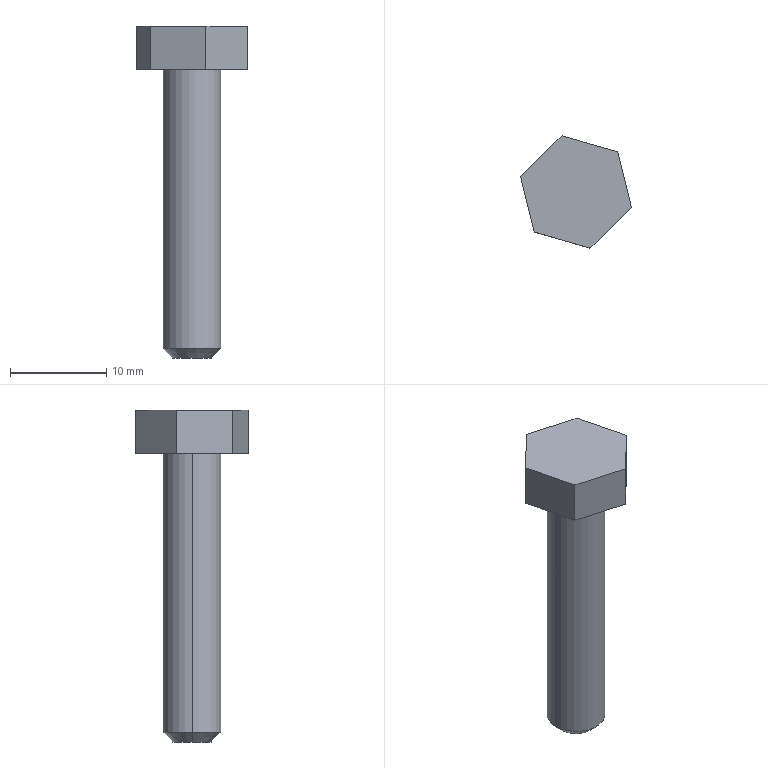Part | SolidWorks | features ICE 2, Chamfer 1, Extrusion 1 | 1 solid | 13 faces | box 11.534 x 11.645 x 34.5 mm | volume 1261 mm3 | plane 9 | cone 2 | cylinder 2 | commonest cylinder face diameters 6 x2
STEP:
#1=CARTESIAN_POINT('',(-2.,0.,-30.));
#2=VERTEX_POINT('',#1);
#3=CARTESIAN_POINT('',(2.,0.,-30.));
#4=VERTEX_POINT('',#3);
#5=CARTESIAN_POINT('',(0.,0.,-30.));
#6=DIRECTION('',(0.,0.,-1.));
#7=DIRECTION('',(-1.,0.,0.));
#8=AXIS2_PLACEMENT_3D('',#5,#6,#7);
#9=CIRCLE('',#8,2.);
#10=EDGE_CURVE('',#2,#4,#9,.T.);
#11=ORIENTED_EDGE('',*,*,#10,.F.);
#12=CARTESIAN_POINT('',(-3.,0.,-29.));
#13=VERTEX_POINT('',#12);
#14=CARTESIAN_POINT('',(-2.,0.,-30.));
#15=DIRECTION('',(-0.7071,0.,0.7071));
#16=VECTOR('',#15,1000.);
#17=LINE('',#14,#16);
#18=EDGE_CURVE('',#2,#13,#17,.T.);
#19=ORIENTED_EDGE('',*,*,#18,.T.);
#20=CARTESIAN_POINT('',(3.,0.,-29.));
#21=VERTEX_POINT('',#20);
#22=CARTESIAN_POINT('',(0.,0.,-29.));
#23=DIRECTION('',(0.,0.,1.));
#24=DIRECTION('',(-1.,0.,0.));
#25=AXIS2_PLACEMENT_3D('',#22,#23,#24);
#26=CIRCLE('',#25,3.);
#27=EDGE_CURVE('',#21,#13,#26,.T.);
#28=ORIENTED_EDGE('',*,*,#27,.F.);
#29=CARTESIAN_POINT('',(2.,0.,-30.));
#30=DIRECTION('',(0.7071,0.,0.7071));
#31=VECTOR('',#30,1000.);
#32=LINE('',#29,#31);
#33=EDGE_CURVE('',#4,#21,#32,.T.);
#34=ORIENTED_EDGE('',*,*,#33,.F.);
#35=EDGE_LOOP('',(#11,#19,#28,#34));
#36=FACE_OUTER_BOUND('',#35,.T.);
#37=CARTESIAN_POINT('',(0.,0.,-30.));
#38=DIRECTION('',(0.,0.,1.));
#39=DIRECTION('',(1.,0.,0.));
#40=AXIS2_PLACEMENT_3D('',#37,#38,#39);
#41=CONICAL_SURFACE('',#40,2.,0.7854);
#42=ADVANCED_FACE('',(#36),#41,.T.);
#43=ORIENTED_EDGE('',*,*,#27,.T.);
#44=CARTESIAN_POINT('',(-3.,0.,0.));
#45=VERTEX_POINT('',#44);
#46=CARTESIAN_POINT('',(-3.,0.,-30.));
#47=DIRECTION('',(0.,0.,1.));
#48=VECTOR('',#47,1000.);
#49=LINE('',#46,#48);
#50=EDGE_CURVE('',#13,#45,#49,.T.);
#51=ORIENTED_EDGE('',*,*,#50,.T.);
#52=CARTESIAN_POINT('',(3.,0.,0.));
#53=VERTEX_POINT('',#52);
#54=CARTESIAN_POINT('',(0.,0.,0.));
#55=DIRECTION('',(0.,0.,-1.));
#56=DIRECTION('',(-1.,0.,0.));
#57=AXIS2_PLACEMENT_3D('',#54,#55,#56);
#58=CIRCLE('',#57,3.);
#59=EDGE_CURVE('',#45,#53,#58,.T.);
#60=ORIENTED_EDGE('',*,*,#59,.T.);
#61=CARTESIAN_POINT('',(3.,0.,-30.));
#62=DIRECTION('',(0.,0.,1.));
#63=VECTOR('',#62,1000.);
#64=LINE('',#61,#63);
#65=EDGE_CURVE('',#21,#53,#64,.T.);
#66=ORIENTED_EDGE('',*,*,#65,.F.);
#67=EDGE_LOOP('',(#43,#51,#60,#66));
#68=FACE_OUTER_BOUND('',#67,.T.);
#69=CARTESIAN_POINT('',(0.,0.,-30.));
#70=DIRECTION('',(0.,0.,1.));
#71=DIRECTION('',(1.,0.,0.));
#72=AXIS2_PLACEMENT_3D('',#69,#70,#71);
#73=CYLINDRICAL_SURFACE('',#72,3.);
#74=ADVANCED_FACE('',(#68),#73,.T.);
#75=CARTESIAN_POINT('',(0.,0.,0.));
#76=DIRECTION('',(0.,0.,-1.));
#77=DIRECTION('',(-1.,0.,0.));
#78=AXIS2_PLACEMENT_3D('',#75,#76,#77);
#79=CIRCLE('',#78,3.);
#80=EDGE_CURVE('',#53,#45,#79,.T.);
#81=ORIENTED_EDGE('',*,*,#80,.F.);
#82=ORIENTED_EDGE('',*,*,#59,.F.);
#83=EDGE_LOOP('',(#81,#82));
#84=FACE_BOUND('',#83,.T.);
#85=CARTESIAN_POINT('',(1.449,-5.822,0.));
#86=VERTEX_POINT('',#85);
#87=CARTESIAN_POINT('',(-4.318,-4.166,0.));
#88=VERTEX_POINT('',#87);
#89=CARTESIAN_POINT('',(1.449,-5.822,0.));
#90=DIRECTION('',(-0.9612,0.276,0.));
#91=VECTOR('',#90,1000.);
#92=LINE('',#89,#91);
#93=EDGE_CURVE('',#86,#88,#92,.T.);
#94=ORIENTED_EDGE('',*,*,#93,.T.);
#95=CARTESIAN_POINT('',(-5.767,1.656,0.));
#96=VERTEX_POINT('',#95);
#97=CARTESIAN_POINT('',(-4.318,-4.166,0.));
#98=DIRECTION('',(-0.2416,0.9704,0.));
#99=VECTOR('',#98,1000.);
#100=LINE('',#97,#99);
#101=EDGE_CURVE('',#88,#96,#100,.T.);
#102=ORIENTED_EDGE('',*,*,#101,.T.);
#103=CARTESIAN_POINT('',(-1.449,5.822,0.));
#104=VERTEX_POINT('',#103);
#105=CARTESIAN_POINT('',(-5.767,1.656,0.));
#106=DIRECTION('',(0.7196,0.6944,0.));
#107=VECTOR('',#106,1000.);
#108=LINE('',#105,#107);
#109=EDGE_CURVE('',#96,#104,#108,.T.);
#110=ORIENTED_EDGE('',*,*,#109,.T.);
#111=CARTESIAN_POINT('',(4.318,4.166,0.));
#112=VERTEX_POINT('',#111);
#113=CARTESIAN_POINT('',(-1.449,5.822,0.));
#114=DIRECTION('',(0.9612,-0.276,0.));
#115=VECTOR('',#114,1000.);
#116=LINE('',#113,#115);
#117=EDGE_CURVE('',#104,#112,#116,.T.);
#118=ORIENTED_EDGE('',*,*,#117,.T.);
#119=CARTESIAN_POINT('',(5.767,-1.656,0.));
#120=VERTEX_POINT('',#119);
#121=CARTESIAN_POINT('',(4.318,4.166,0.));
#122=DIRECTION('',(0.2416,-0.9704,0.));
#123=VECTOR('',#122,1000.);
#124=LINE('',#121,#123);
#125=EDGE_CURVE('',#112,#120,#124,.T.);
#126=ORIENTED_EDGE('',*,*,#125,.T.);
#127=CARTESIAN_POINT('',(5.767,-1.656,0.));
#128=DIRECTION('',(-0.7196,-0.6944,0.));
#129=VECTOR('',#128,1000.);
#130=LINE('',#127,#129);
#131=EDGE_CURVE('',#120,#86,#130,.T.);
#132=ORIENTED_EDGE('',*,*,#131,.T.);
#133=EDGE_LOOP('',(#94,#102,#110,#118,#126,#132));
#134=FACE_OUTER_BOUND('',#133,.T.);
#135=CARTESIAN_POINT('',(0.,0.,0.));
#136=DIRECTION('',(0.,0.,1.));
#137=DIRECTION('',(1.,0.,0.));
#138=AXIS2_PLACEMENT_3D('',#135,#136,#137);
#139=PLANE('',#138);
#140=ADVANCED_FACE('',(#84,#134),#139,.F.);
#141=ORIENTED_EDGE('',*,*,#93,.F.);
#142=CARTESIAN_POINT('',(1.449,-5.822,4.5));
#143=VERTEX_POINT('',#142);
#144=CARTESIAN_POINT('',(1.449,-5.822,4.5));
#145=DIRECTION('',(0.,0.,-1.));
#146=VECTOR('',#145,1000.);
#147=LINE('',#144,#146);
#148=EDGE_CURVE('',#143,#86,#147,.T.);
#149=ORIENTED_EDGE('',*,*,#148,.F.);
#150=CARTESIAN_POINT('',(-4.318,-4.166,4.5));
#151=VERTEX_POINT('',#150);
#152=CARTESIAN_POINT('',(1.449,-5.822,4.5));
#153=DIRECTION('',(-0.9612,0.276,0.));
#154=VECTOR('',#153,1000.);
#155=LINE('',#152,#154);
#156=EDGE_CURVE('',#143,#151,#155,.T.);
#157=ORIENTED_EDGE('',*,*,#156,.T.);
#158=CARTESIAN_POINT('',(-4.318,-4.166,4.5));
#159=DIRECTION('',(0.,0.,-1.));
#160=VECTOR('',#159,1000.);
#161=LINE('',#158,#160);
#162=EDGE_CURVE('',#151,#88,#161,.T.);
#163=ORIENTED_EDGE('',*,*,#162,.T.);
#164=EDGE_LOOP('',(#141,#149,#157,#163));
#165=FACE_OUTER_BOUND('',#164,.T.);
#166=CARTESIAN_POINT('',(1.449,-5.822,4.5));
#167=DIRECTION('',(-0.276,-0.9612,0.));
#168=DIRECTION('',(0.9612,-0.276,0.));
#169=AXIS2_PLACEMENT_3D('',#166,#167,#168);
#170=PLANE('',#169);
#171=ADVANCED_FACE('',(#165),#170,.T.);
#172=ORIENTED_EDGE('',*,*,#131,.F.);
#173=CARTESIAN_POINT('',(5.767,-1.656,4.5));
#174=VERTEX_POINT('',#173);
#175=CARTESIAN_POINT('',(5.767,-1.656,4.5));
#176=DIRECTION('',(0.,0.,-1.));
#177=VECTOR('',#176,1000.);
#178=LINE('',#175,#177);
#179=EDGE_CURVE('',#174,#120,#178,.T.);
#180=ORIENTED_EDGE('',*,*,#179,.F.);
#181=CARTESIAN_POINT('',(5.767,-1.656,4.5));
#182=DIRECTION('',(-0.7196,-0.6944,0.));
#183=VECTOR('',#182,1000.);
#184=LINE('',#181,#183);
#185=EDGE_CURVE('',#174,#143,#184,.T.);
#186=ORIENTED_EDGE('',*,*,#185,.T.);
#187=ORIENTED_EDGE('',*,*,#148,.T.);
#188=EDGE_LOOP('',(#172,#180,#186,#187));
#189=FACE_OUTER_BOUND('',#188,.T.);
#190=CARTESIAN_POINT('',(5.767,-1.656,4.5));
#191=DIRECTION('',(0.6944,-0.7196,0.));
#192=DIRECTION('',(0.7196,0.6944,0.));
#193=AXIS2_PLACEMENT_3D('',#190,#191,#192);
#194=PLANE('',#193);
#195=ADVANCED_FACE('',(#189),#194,.T.);
#196=ORIENTED_EDGE('',*,*,#125,.F.);
#197=CARTESIAN_POINT('',(4.318,4.166,4.5));
#198=VERTEX_POINT('',#197);
#199=CARTESIAN_POINT('',(4.318,4.166,4.5));
#200=DIRECTION('',(0.,0.,-1.));
#201=VECTOR('',#200,1000.);
#202=LINE('',#199,#201);
#203=EDGE_CURVE('',#198,#112,#202,.T.);
#204=ORIENTED_EDGE('',*,*,#203,.F.);
#205=CARTESIAN_POINT('',(4.318,4.166,4.5));
#206=DIRECTION('',(0.2416,-0.9704,0.));
#207=VECTOR('',#206,1000.);
#208=LINE('',#205,#207);
#209=EDGE_CURVE('',#198,#174,#208,.T.);
#210=ORIENTED_EDGE('',*,*,#209,.T.);
#211=ORIENTED_EDGE('',*,*,#179,.T.);
#212=EDGE_LOOP('',(#196,#204,#210,#211));
#213=FACE_OUTER_BOUND('',#212,.T.);
#214=CARTESIAN_POINT('',(4.318,4.166,4.5));
#215=DIRECTION('',(0.9704,0.2416,0.));
#216=DIRECTION('',(-0.2416,0.9704,0.));
#217=AXIS2_PLACEMENT_3D('',#214,#215,#216);
#218=PLANE('',#217);
#219=ADVANCED_FACE('',(#213),#218,.T.);
#220=ORIENTED_EDGE('',*,*,#117,.F.);
#221=CARTESIAN_POINT('',(-1.449,5.822,4.5));
#222=VERTEX_POINT('',#221);
#223=CARTESIAN_POINT('',(-1.449,5.822,4.5));
#224=DIRECTION('',(0.,0.,-1.));
#225=VECTOR('',#224,1000.);
#226=LINE('',#223,#225);
#227=EDGE_CURVE('',#222,#104,#226,.T.);
#228=ORIENTED_EDGE('',*,*,#227,.F.);
#229=CARTESIAN_POINT('',(-1.449,5.822,4.5));
#230=DIRECTION('',(0.9612,-0.276,0.));
#231=VECTOR('',#230,1000.);
#232=LINE('',#229,#231);
#233=EDGE_CURVE('',#222,#198,#232,.T.);
#234=ORIENTED_EDGE('',*,*,#233,.T.);
#235=ORIENTED_EDGE('',*,*,#203,.T.);
#236=EDGE_LOOP('',(#220,#228,#234,#235));
#237=FACE_OUTER_BOUND('',#236,.T.);
#238=CARTESIAN_POINT('',(-1.449,5.822,4.5));
#239=DIRECTION('',(0.276,0.9612,0.));
#240=DIRECTION('',(-0.9612,0.276,0.));
#241=AXIS2_PLACEMENT_3D('',#238,#239,#240);
#242=PLANE('',#241);
#243=ADVANCED_FACE('',(#237),#242,.T.);
#244=ORIENTED_EDGE('',*,*,#109,.F.);
#245=CARTESIAN_POINT('',(-5.767,1.656,4.5));
#246=VERTEX_POINT('',#245);
#247=CARTESIAN_POINT('',(-5.767,1.656,4.5));
#248=DIRECTION('',(0.,0.,-1.));
#249=VECTOR('',#248,1000.);
#250=LINE('',#247,#249);
#251=EDGE_CURVE('',#246,#96,#250,.T.);
#252=ORIENTED_EDGE('',*,*,#251,.F.);
#253=CARTESIAN_POINT('',(-5.767,1.656,4.5));
#254=DIRECTION('',(0.7196,0.6944,0.));
#255=VECTOR('',#254,1000.);
#256=LINE('',#253,#255);
#257=EDGE_CURVE('',#246,#222,#256,.T.);
#258=ORIENTED_EDGE('',*,*,#257,.T.);
#259=ORIENTED_EDGE('',*,*,#227,.T.);
#260=EDGE_LOOP('',(#244,#252,#258,#259));
#261=FACE_OUTER_BOUND('',#260,.T.);
#262=CARTESIAN_POINT('',(-5.767,1.656,4.5));
#263=DIRECTION('',(-0.6944,0.7196,0.));
#264=DIRECTION('',(-0.7196,-0.6944,0.));
#265=AXIS2_PLACEMENT_3D('',#262,#263,#264);
#266=PLANE('',#265);
#267=ADVANCED_FACE('',(#261),#266,.T.);
#268=ORIENTED_EDGE('',*,*,#101,.F.);
#269=ORIENTED_EDGE('',*,*,#162,.F.);
#270=CARTESIAN_POINT('',(-4.318,-4.166,4.5));
#271=DIRECTION('',(-0.2416,0.9704,0.));
#272=VECTOR('',#271,1000.);
#273=LINE('',#270,#272);
#274=EDGE_CURVE('',#151,#246,#273,.T.);
#275=ORIENTED_EDGE('',*,*,#274,.T.);
#276=ORIENTED_EDGE('',*,*,#251,.T.);
#277=EDGE_LOOP('',(#268,#269,#275,#276));
#278=FACE_OUTER_BOUND('',#277,.T.);
#279=CARTESIAN_POINT('',(-4.318,-4.166,4.5));
#280=DIRECTION('',(-0.9704,-0.2416,0.));
#281=DIRECTION('',(0.2416,-0.9704,0.));
#282=AXIS2_PLACEMENT_3D('',#279,#280,#281);
#283=PLANE('',#282);
#284=ADVANCED_FACE('',(#278),#283,.T.);
#285=ORIENTED_EDGE('',*,*,#274,.F.);
#286=ORIENTED_EDGE('',*,*,#156,.F.);
#287=ORIENTED_EDGE('',*,*,#185,.F.);
#288=ORIENTED_EDGE('',*,*,#209,.F.);
#289=ORIENTED_EDGE('',*,*,#233,.F.);
#290=ORIENTED_EDGE('',*,*,#257,.F.);
#291=EDGE_LOOP('',(#285,#286,#287,#288,#289,#290));
#292=FACE_OUTER_BOUND('',#291,.T.);
#293=CARTESIAN_POINT('',(0.,0.,4.5));
#294=DIRECTION('',(0.,0.,1.));
#295=DIRECTION('',(1.,0.,0.));
#296=AXIS2_PLACEMENT_3D('',#293,#294,#295);
#297=PLANE('',#296);
#298=ADVANCED_FACE('',(#292),#297,.T.);
#299=ORIENTED_EDGE('',*,*,#50,.F.);
#300=CARTESIAN_POINT('',(0.,0.,-29.));
#301=DIRECTION('',(0.,0.,1.));
#302=DIRECTION('',(-1.,0.,0.));
#303=AXIS2_PLACEMENT_3D('',#300,#301,#302);
#304=CIRCLE('',#303,3.);
#305=EDGE_CURVE('',#13,#21,#304,.T.);
#306=ORIENTED_EDGE('',*,*,#305,.T.);
#307=ORIENTED_EDGE('',*,*,#65,.T.);
#308=ORIENTED_EDGE('',*,*,#80,.T.);
#309=EDGE_LOOP('',(#299,#306,#307,#308));
#310=FACE_OUTER_BOUND('',#309,.T.);
#311=CARTESIAN_POINT('',(0.,0.,-30.));
#312=DIRECTION('',(0.,0.,1.));
#313=DIRECTION('',(1.,0.,0.));
#314=AXIS2_PLACEMENT_3D('',#311,#312,#313);
#315=CYLINDRICAL_SURFACE('',#314,3.);
#316=ADVANCED_FACE('',(#310),#315,.T.);
#317=CARTESIAN_POINT('',(0.,0.,-30.));
#318=DIRECTION('',(0.,0.,-1.));
#319=DIRECTION('',(-1.,0.,0.));
#320=AXIS2_PLACEMENT_3D('',#317,#318,#319);
#321=CIRCLE('',#320,2.);
#322=EDGE_CURVE('',#4,#2,#321,.T.);
#323=ORIENTED_EDGE('',*,*,#322,.T.);
#324=ORIENTED_EDGE('',*,*,#10,.T.);
#325=EDGE_LOOP('',(#323,#324));
#326=FACE_OUTER_BOUND('',#325,.T.);
#327=CARTESIAN_POINT('',(0.,0.,-30.));
#328=DIRECTION('',(0.,0.,-1.));
#329=DIRECTION('',(-1.,0.,0.));
#330=AXIS2_PLACEMENT_3D('',#327,#328,#329);
#331=PLANE('',#330);
#332=ADVANCED_FACE('',(#326),#331,.T.);
#333=ORIENTED_EDGE('',*,*,#18,.F.);
#334=ORIENTED_EDGE('',*,*,#322,.F.);
#335=ORIENTED_EDGE('',*,*,#33,.T.);
#336=ORIENTED_EDGE('',*,*,#305,.F.);
#337=EDGE_LOOP('',(#333,#334,#335,#336));
#338=FACE_OUTER_BOUND('',#337,.T.);
#339=CARTESIAN_POINT('',(0.,0.,-30.));
#340=DIRECTION('',(0.,0.,1.));
#341=DIRECTION('',(1.,0.,0.));
#342=AXIS2_PLACEMENT_3D('',#339,#340,#341);
#343=CONICAL_SURFACE('',#342,2.,0.7854);
#344=ADVANCED_FACE('',(#338),#343,.T.);
#345=CLOSED_SHELL('',(#42,#74,#140,#171,#195,#219,#243,#267,#284,#298,#316,#332,#344));
#346=MANIFOLD_SOLID_BREP('',#345);
#347=CARTESIAN_POINT('',(0.,0.,0.));
#348=DIRECTION('',(0.,0.,1.));
#349=DIRECTION('',(1.,0.,0.));
#350=AXIS2_PLACEMENT_3D('',#347,#348,#349);
#351=(LENGTH_UNIT()NAMED_UNIT(*)SI_UNIT(.MILLI.,.METRE.));
#352=UNCERTAINTY_MEASURE_WITH_UNIT(LENGTH_MEASURE(0.00001),#351,'','');
#353=(NAMED_UNIT(*)PLANE_ANGLE_UNIT()SI_UNIT($,.RADIAN.));
#354=(NAMED_UNIT(*)SI_UNIT($,.STERADIAN.)SOLID_ANGLE_UNIT());
#355=(GEOMETRIC_REPRESENTATION_CONTEXT(3)GLOBAL_UNCERTAINTY_ASSIGNED_CONTEXT((#352))GLOBAL_UNIT_ASSIGNED_CONTEXT((#351,#353,#354))REPRESENTATION_CONTEXT('',''));
#356=ADVANCED_BREP_SHAPE_REPRESENTATION('',(#346,#350),#355);